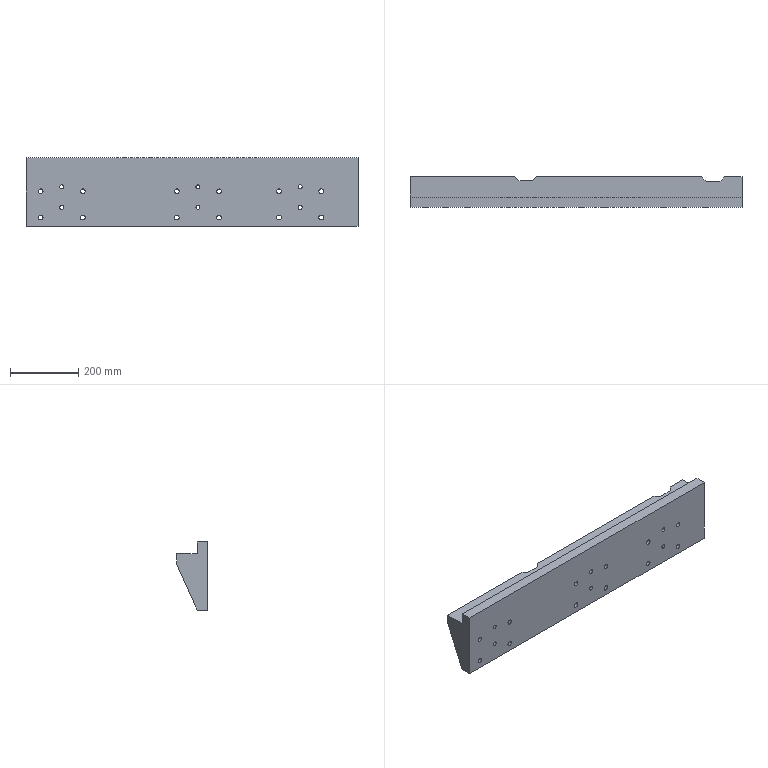Part | NX | features solid 2 | 1 solid | 74 faces | box 975 x 90 x 200 mm | volume 7934348 mm3 | plane 44 | cylinder 30 | commonest cylinder face diameters 14 x12 20 x12 12 x6